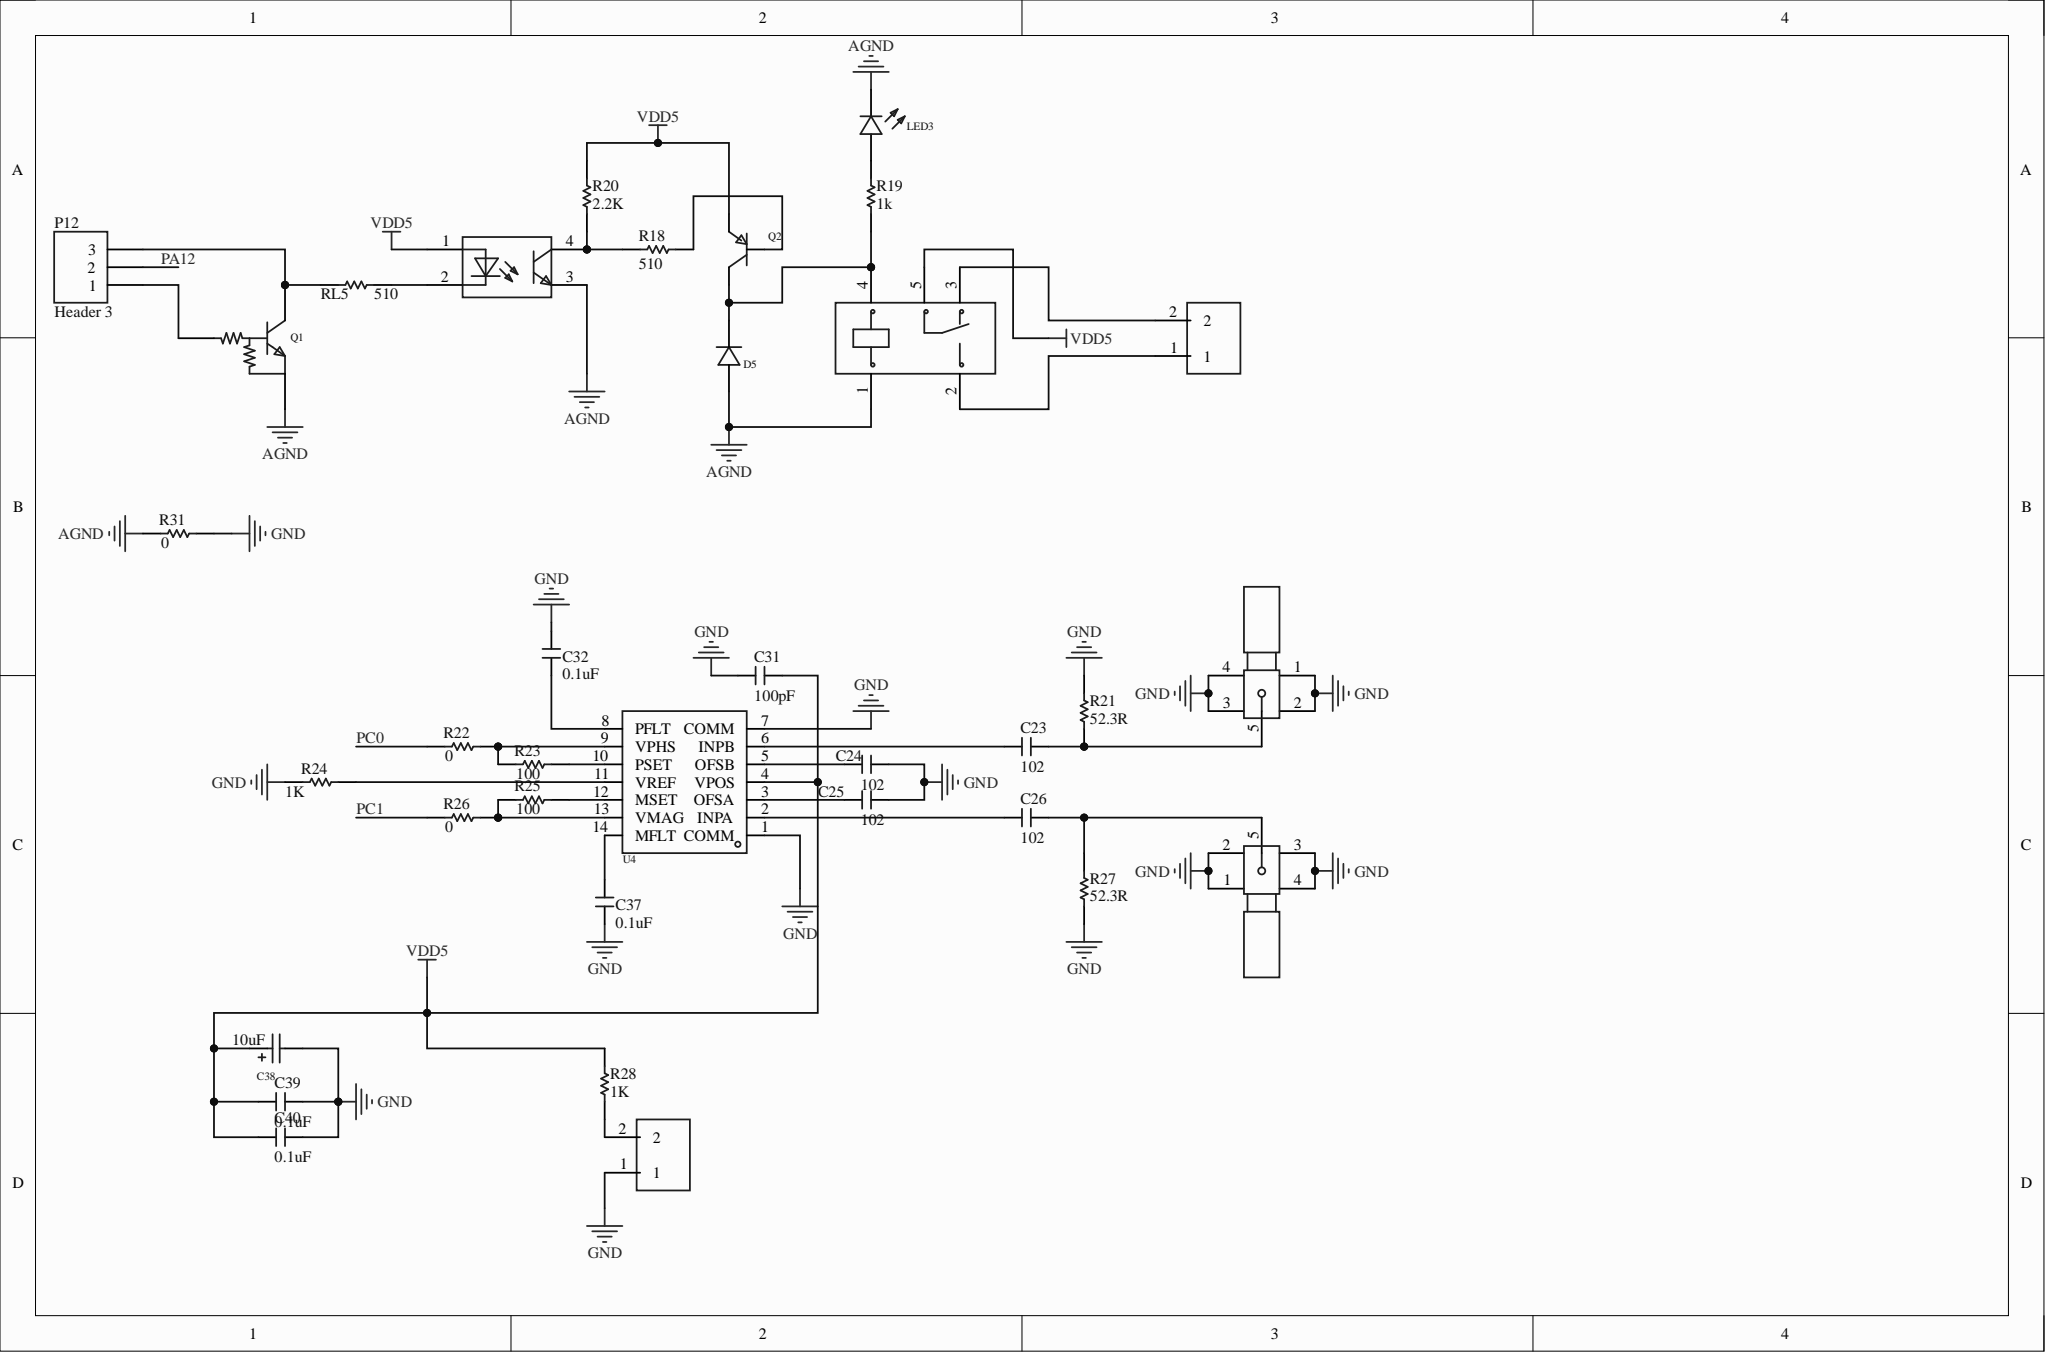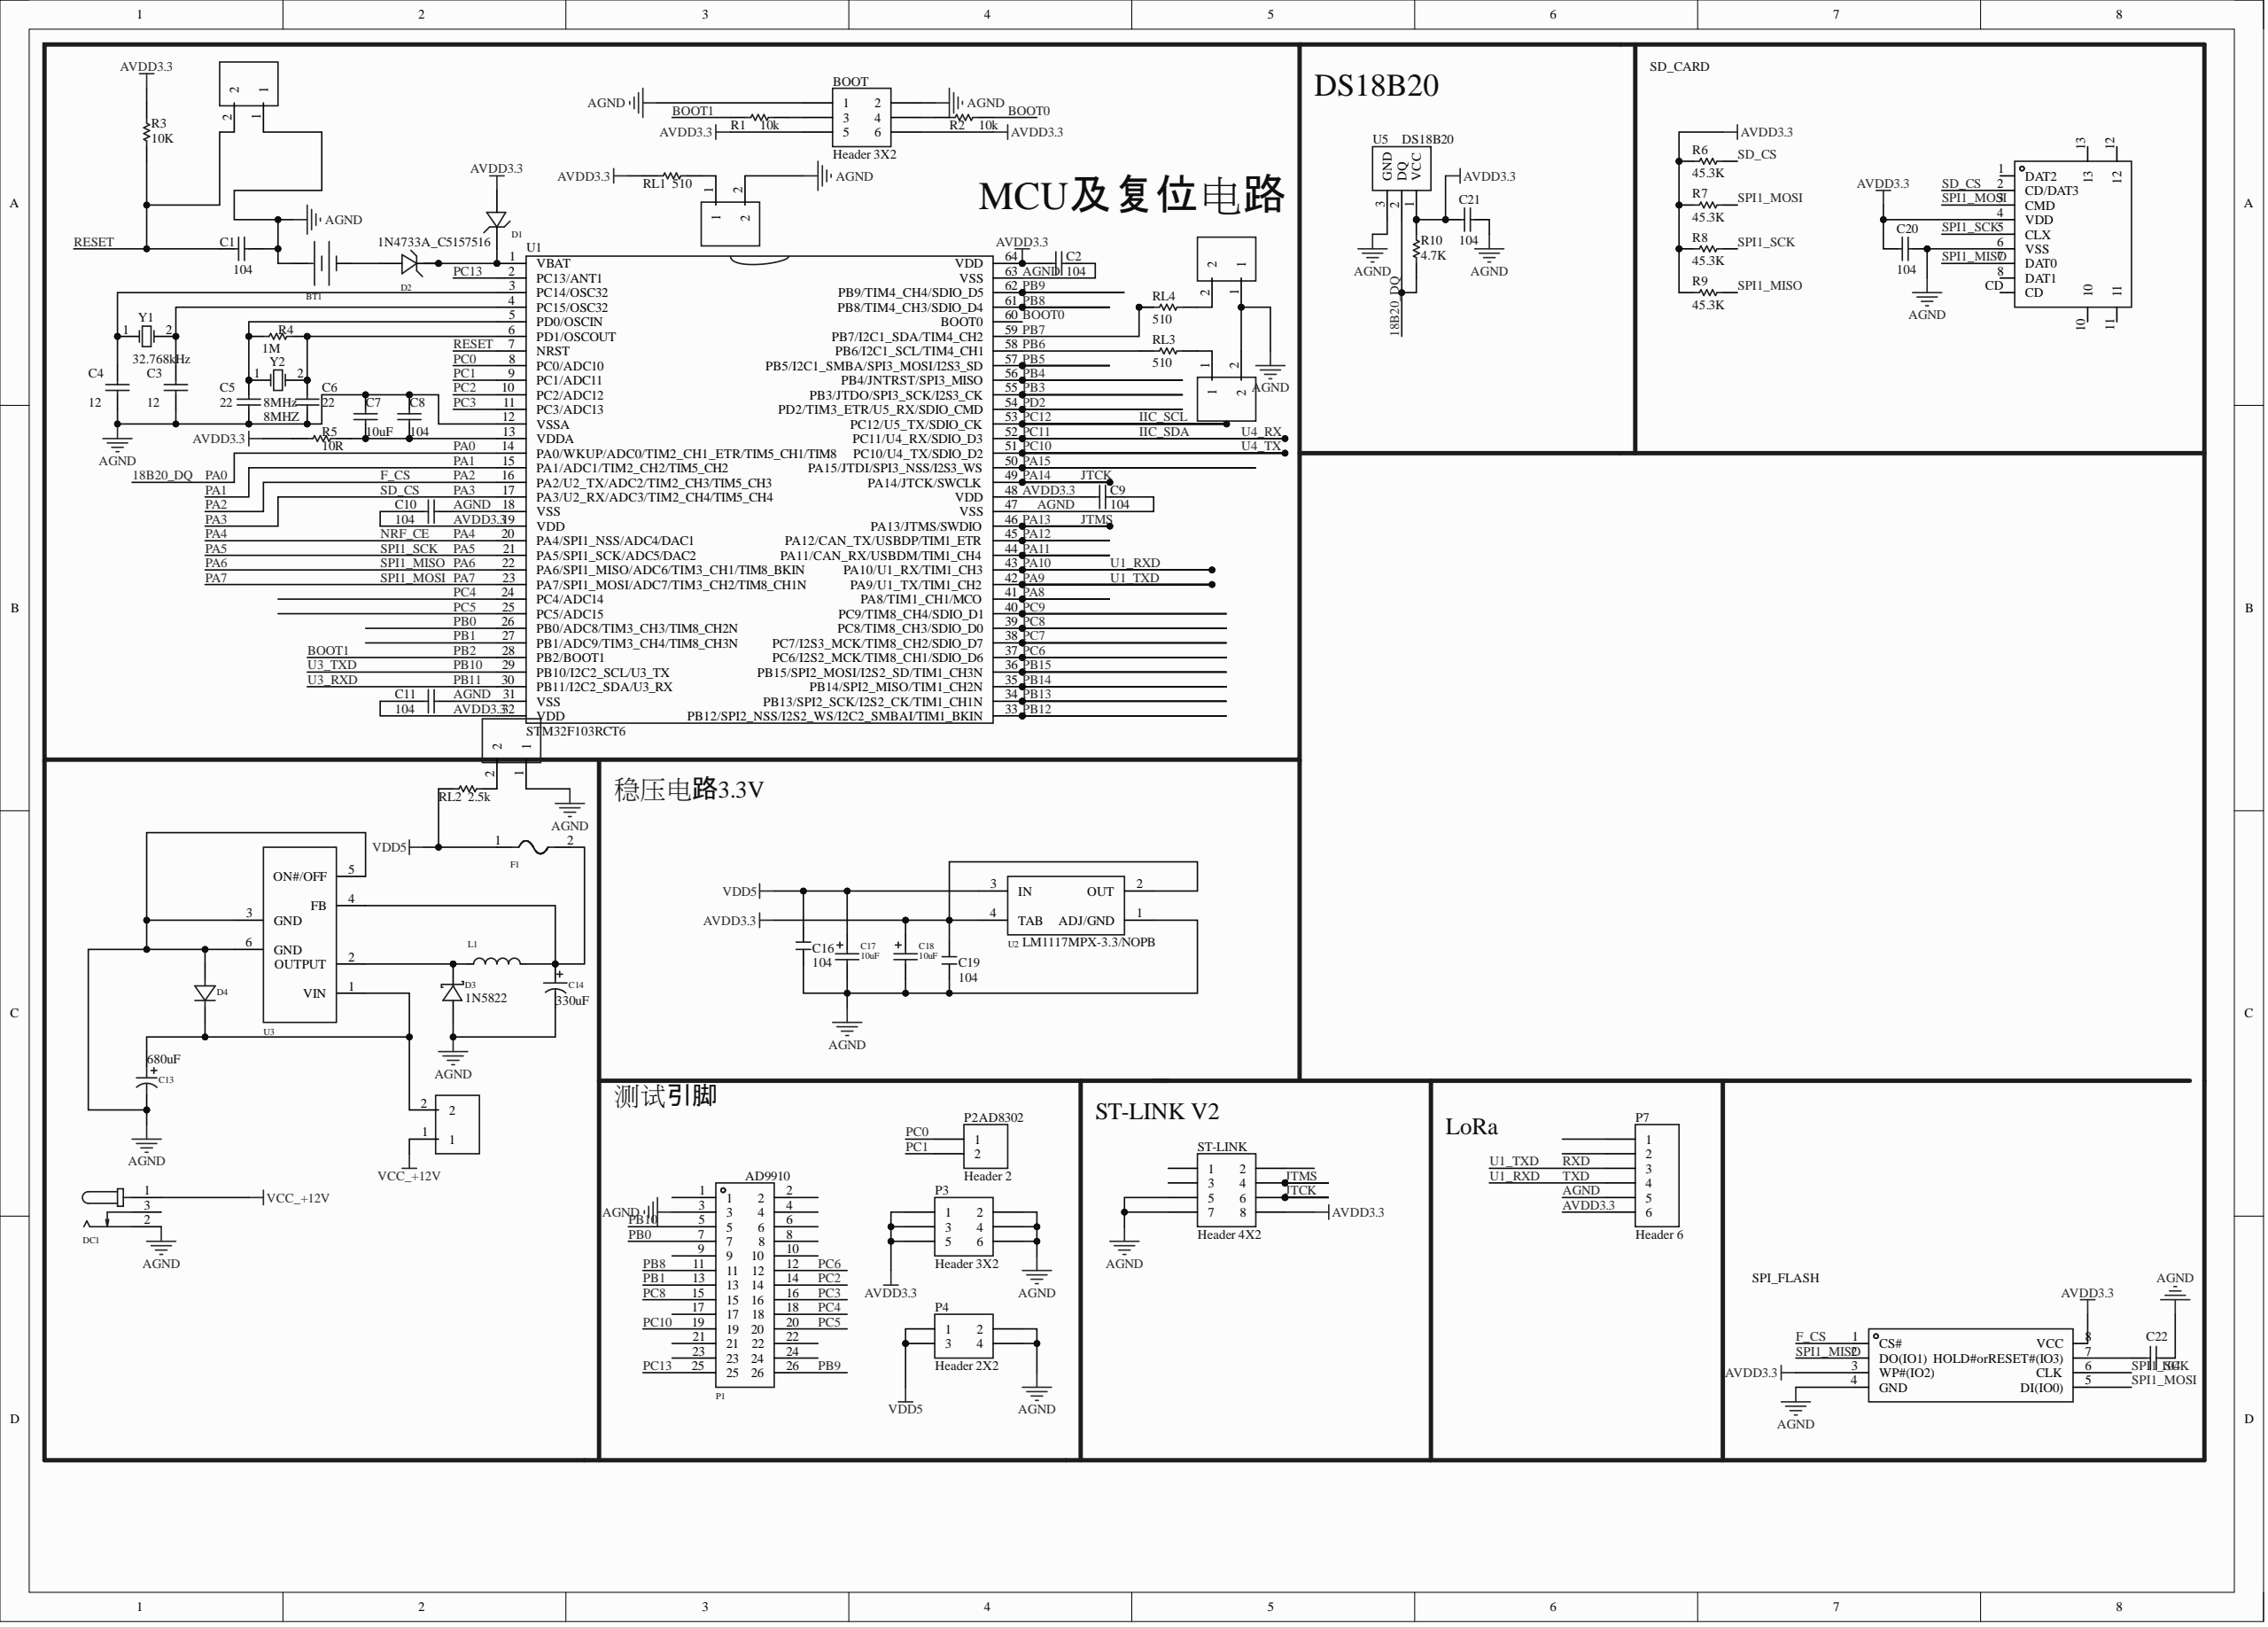Circuit board | Altium Designer | 98 parts | 76 nets
Bill of materials:
Comment,Description,Designator,Footprint,LibRef,Quantity
"Header 3X2","Header, 3-Pin, Dual row","BOOT, P3","HDR2X3","Header 3X2, Header 3X2_1","2"
"BS-12-B3AA003","","BT1","BAT-SMD_BS-12-B3AA011","BS-12-B3AA003","1"
"104","104","C1, C2, C8, C9, C10, C11, C16, C19","C0603","104, 104_1","8"
"12pF","12pF","C3, C4","C0603","12pF","2"
"22pF","22pF","C5, C6","C0603","22pF","2"
"10uF","10uF","C7","C0603","10uF","1"
"GVM1V681M1010","680uF","C13","CAP-SMD_BD10.0-L10.3-W10.3-LS10.9-FD","GVM1V681M1010","1"
"EEEFK1V331P","330uF","C14","CAP-SMD_BD10.0-L10.3-W10.3-FD","EEEFK1V331P","1"
"TAJA106K016RNJ","10uF","C17, C18","CAP-SMD_L3.2-W1.6-RD-C7171","TAJA106K016RNJ","2"
"Cap","104, Cap","C20, C21, C22","CAP[0603]","Cap","3"
"102","102","C23, C24, C25, C26","C0603","102","4"
"100pF","100pF","C31","C0603","100pF","1"
"0.1uF","0.1uF","C32, C37, C39, C40","C0603","0.1uF","4"
"10uF","10uF","C38","CAP-SMD_L3.2-W1.6-RD-C7171","10uF_1","1"
"TF PUSH","","CARD","TF-SMD_TF-PUSH","TF PUSH","1"
"1N4733A_C5157516","","D1, D2","DO-41_BD2.4-L4.7-P8.70-D0.9-RD","1N4733A_C5157516","2"
"1N5822","","D3","DO-201AD_BD5.3-L8.4-P12.50-D1.4-FD","1N5822","1"
"1N4007_C727081","","D4","SMA_L4.3-W2.5-LS5.0-RD","1N4007_C727081","1"
"1N4007W","","D5","SOD-123FL_L2.7-W1.8-LS3.8-RD","1N4007W","1"
"DC-005-20A_C136744","","DC1","DC-IN-TH_DC-005-20A","DC-005-20A_C136744","1"
"BSMD1812-150-33V","","F1","F1812","BSMD1812-150-33V","1"
"FXL0650-330-M","","L1","IND-SMD_L7.0-W6.6_FXL0650","FXL0650-330-M","1"
"NCD0603R1_C84263","","LED3","LED0603-RD_RED","NCD0603R1_C84263","1"
"X1270WV-2x13A-6TV01","","P1","IDC-TH_X1270WV-2X13A-6TV01","X1270WV-2x13A-6TV01","1"
"Header 2","Header, 2-Pin","P2","HDR1X2","Header 2","1"
"Header 2X2","Header, 2-Pin, Dual row","P4","HDR2X2","Header 2X2","1"
"Header 6","Header, 6-Pin","P7","HDR1X6","Header 6","1"
"Header 3","Header, 3-Pin","P12","HDR1X3","Header 3","1"
"WJ126V-5.0-2P","","P13, P17, P18, P19, P20, P21, P22, P23","CONN-TH_WJ126V-5.0-2P","WJ126V-5.0-2P_1, WJ126V-5.0-2P","8"
"DTC143ECA","","Q1","SOT-23-3_L2.9-W1.6-P1.90-LS2.8-BR","DTC143ECA","1"
"MMBT3906","","Q2","SOT-23-3_L2.9-W1.3-P1.90-LS2.4-BR","MMBT3906","1"
"10k","10K, Res","R1, R18, R19, R20","R0603 - duplicate","10k_1","4"
"10k","10K","R2, R3","R0603","10k","2"
"1M","Res","R4","R0603","1M","1"
"10R","10","R5","R0603","10R","1"
"Res","45.3K, 4.7K","R6, R7, R8, R9, R10","RES[0603]","Res","5"
"52.3R","52.3R","R21, R27","R0603","52.3R","2"
"0","0","R22, R26, R31","R0603","0","3"
"100","100","R23, R25","R0603","100","2"
"1K","1K","R24, R28","R0603","1K","2"
"BWSMA-KWE-Z001","","RF1, RF?1","SMA-TH_BWSMA-KWE-Z001","BWSMA-KWE-Z001_1, BWSMA-KWE-Z001","2"
"330","510, 2.5K, Res","RL1, RL2, RL3, RL4, RL5","R0603 - duplicate","330","5"
"SRD-05VDC-SL-C","","RLY1","RELAY-TH_SRD-XXVDC-XL-C","SRD-05VDC-SL-C","1"
"Header 4X2","Header, 4-Pin, Dual row","ST-LINK","HDR2X4","Header 4X2","1"
"STM32F103RCT6","","U1","TQFP-64_L10.0-W10.0-P0.50-LS12.0-BL","STM32F103RCT6","1"
"LM1117MPX-3.3/NOPB","","U2","SOT-223-3_L6.5-W3.4-P2.30-LS7.0-BR","LM1117MPX-3.3/NOPB","1"
"LM2596SX-5.0/NOPB","","U3","TO-263-5_L10.2-W8.9-P1.70-TL","LM2596SX-5.0/NOPB","1"
"AD8302ARUZ-RL7","","U4","TSSOP-14_L5.0-W4.4-P0.65-LS6.4-BL","AD8302ARUZ-RL7","1"
"DS18B20","DS18B20","U5","H2.54-1X3(RM)","DS18B20","1"
"BPC-817SC","","U6","OPTO-SMD-4_L4.6-W6.5-P2.54-LS10.3-BR","BPC-817SC","1"
"W25Q64JVSSIQ","","W25Q64","SOIC-8_L5.3-W5.3-P1.27-LS8.0-BL","W25Q64JVSSIQ","1"
"32.768kHz","XTAL","Y1","OSC-TH_BD2.0-P0.70-D0.3","32.768kHz","1"
"8MHz","XTAL","Y2","OSC-TH_L11.1-W4.7-P4.88","8MHz","1"
Netlist (Protel format):
[
BOOT
HDR2X3
Header 3X2



]
[
BT1
BAT-SMD_BS-12-B3AA011
BS-12-B3AA003



]
[
C1
C0603
104



]
[
C2
C0603
104



]
[
C3
C0603
12pF



]
[
C4
C0603
12pF



]
[
C5
C0603
22pF



]
[
C6
C0603
22pF



]
[
C7
C0603
10uF



]
[
C8
C0603
104



]
[
C9
C0603
104



]
[
C10
C0603
104



]
[
C11
C0603
104



]
[
C13
CAP-SMD_BD10.0-L10.3-W10.3-LS10.9-FD
GVM1V681M1010



]
[
C14
CAP-SMD_BD10.0-L10.3-W10.3-FD
EEEFK1V331P



]
[
C16
C0603
104



]
[
C17
CAP-SMD_L3.2-W1.6-RD-C7171
TAJA106K016RNJ



]
[
C18
CAP-SMD_L3.2-W1.6-RD-C7171
TAJA106K016RNJ



]
[
C19
C0603
104



]
[
C20
CAP[0603]
Cap



]
[
C21
CAP[0603]
Cap



]
[
C22
CAP[0603]
Cap



]
[
C23
C0603
102



]
[
C24
C0603
102



]
[
C25
C0603
102



]
[
C26
C0603
102



]
[
C31
C0603
100pF



]
[
C32
C0603
0.1uF



]
[
C37
C0603
0.1uF



]
[
C38
CAP-SMD_L3.2-W1.6-RD-C7171
10uF



]
[
C39
C0603
0.1uF



]
[
C40
C0603
0.1uF



]
[
CARD
TF-SMD_TF-PUSH
TF PUSH



]
[
D1
DO-41_BD2.4-L4.7-P8.70-D0.9-RD
1N4733A_C5157516



]
[
D2
DO-41_BD2.4-L4.7-P8.70-D0.9-RD
1N4733A_C5157516



]
[
D3
DO-201AD_BD5.3-L8.4-P12.50-D1.4-FD
1N5822



]
[
D4
SMA_L4.3-W2.5-LS5.0-RD
1N4007_C727081



]
[
D5
SOD-123FL_L2.7-W1.8-LS3.8-RD
1N4007W



]
[
DC1
DC-IN-TH_DC-005-20A
DC-005-20A_C136744



]
[
F1
F1812
BSMD1812-150-33V



]
[
L1
IND-SMD_L7.0-W6.6_FXL0650
FXL0650-330-M



]
[
LED3
LED0603-RD_RED
NCD0603R1_C84263



]
[
P1
IDC-TH_X1270WV-2X13A-6TV01
X1270WV-2x13A-6TV01



]
[
P2
HDR1X2
Header 2



]
[
P3
HDR2X3
Header 3X2



]
[
P4
HDR2X2
Header 2X2



]
[
P7
HDR1X6
Header 6



]
[
P12
HDR1X3
Header 3



]
[
P13
CONN-TH_WJ126V-5.0-2P
WJ126V-5.0-2P



]
[
P17
CONN-TH_WJ126V-5.0-2P
WJ126V-5.0-2P



]
[
P18
CONN-TH_WJ126V-5.0-2P
WJ126V-5.0-2P



]
[
P19
CONN-TH_WJ126V-5.0-2P
WJ126V-5.0-2P



]
[
P20
CONN-TH_WJ126V-5.0-2P
WJ126V-5.0-2P



]
[
P21
CONN-TH_WJ126V-5.0-2P
WJ126V-5.0-2P



]
[
P22
CONN-TH_WJ126V-5.0-2P
WJ126V-5.0-2P



]
[
P23
CONN-TH_WJ126V-5.0-2P
WJ126V-5.0-2P



]
[
Q1
SOT-23-3_L2.9-W1.6-P1.90-LS2.8-BR
DTC143ECA



]
[
Q2
SOT-23-3_L2.9-W1.3-P1.90-LS2.4-BR
MMBT3906



]
[
R1
R0603 - duplicate
10k



]
[
R2
R0603
10k



]
[
R3
R0603
10k



]
[
R4
R0603
1M



]
[
R5
R0603
10R



]
[
R6
RES[0603]
Res



]
[
R7
RES[0603]
Res



]
[
R8
RES[0603]
Res



]
[
R9
RES[0603]
Res



]
[
R10
RES[0603]
Res



]
[
R18
R0603 - duplicate
10k



]
[
R19
R0603 - duplicate
10k



]
[
R20
R0603 - duplicate
10k



]
[
R21
R0603
52.3R



]
[
R22
R0603
0



]
[
R23
R0603
100



]
[
R24
R0603
1K



]
[
R25
R0603
100



]
[
R26
R0603
0



]
[
R27
R0603
52.3R



]
[
R28
R0603
1K



]
[
R31
R0603
0



]
[
RF1
SMA-TH_BWSMA-KWE-Z001
BWSMA-KWE-Z001



]
[
RF?1
SMA-TH_BWSMA-KWE-Z001
BWSMA-KWE-Z001



]
[
RL1
R0603 - duplicate
330



]
[
RL2
R0603 - duplicate
330



]
[
RL3
R0603 - duplicate
330



]
[
RL4
R0603 - duplicate
330



]
[
RL5
R0603 - duplicate
330



]
[
RLY1
RELAY-TH_SRD-XXVDC-XL-C
SRD-05VDC-SL-C



]
[
ST-LINK
HDR2X4
Header 4X2



]
[
U1
TQFP-64_L10.0-W10.0-P0.50-LS12.0-BL
STM32F103RCT6



]
[
U2
SOT-223-3_L6.5-W3.4-P2.30-LS7.0-BR
LM1117MPX-3.3/NOPB



]
[
U3
TO-263-5_L10.2-W8.9-P1.70-TL
LM2596SX-5.0/NOPB



]
[
U4
TSSOP-14_L5.0-W4.4-P0.65-LS6.4-BL
AD8302ARUZ-RL7



]
[
U5
H2.54-1X3(RM)
DS18B20



]
[
U6
OPTO-SMD-4_L4.6-W6.5-P2.54-LS10.3-BR
BPC-817SC



]
[
W25Q64
SOIC-8_L5.3-W5.3-P1.27-LS8.0-BL
W25Q64JVSSIQ



]
[
Y1
OSC-TH_BD2.0-P0.70-D0.3
32.768kHz



]
[
Y2
OSC-TH_L11.1-W4.7-P4.88
8MHz



]
(
VDD5
C16-2
C17-1
C31-1
C38-1
C39-2
C40-2
F1-1
P4-1
P4-3
Q2-2
R20-1
R28-2
RL2-1
RLY1-5
U2-3
U4-4
U6-1
)
(
VCC_+12V
DC1-1
P22-1
)
(
RESET
C1-1
P23-2
R3-1
U1-7
)
(
PC13
P1-25
U1-2
)
(
PC10
P1-19
U1-51
)
(
PC8
P1-15
U1-39
)
(
PC6
P1-12
U1-37
)
(
PC5
P1-20
U1-25
)
(
PC4
P1-18
U1-24
)
(
PC3
P1-16
U1-11
)
(
PC2
P1-14
U1-10
)
(
PC1
P2-2
R26-1
U1-9
)
(
PC0
P2-1
R22-1
U1-8
)
(
PB10
P1-5
U1-29
)
(
PB9
P1-26
U1-62
)
(
PB8
P1-11
U1-61
)
(
PB7
RL4-2
U1-59
)
(
PB6
RL3-2
U1-58
)
(
PB1
P1-13
U1-27
)
(
PB0
P1-7
U1-26
)
(
PA12
P12-2
U1-45
)
(
PA10
P7-4
U1-43
)
(
PA9
P7-3
U1-42
)
(
PA7
CARD-3
R7-2
U1-23
W25Q64-5
)
(
PA6
CARD-7
R9-2
U1-22
W25Q64-2
)
(
PA5
CARD-5
R8-2
U1-21
W25Q64-6
)
(
PA3
CARD-2
R6-2
U1-17
)
(
NetRL5_2
RL5-2
U6-2
)
(
NetR25_2
R25-2
U4-12
)
(
NetR25_1
R25-1
R26-2
U4-13
)
(
NetR24_2
R24-2
U4-11
)
(
NetR23_2
R23-2
U4-10
)
(
NetR22_2
R22-2
R23-1
U4-9
)
(
NetR18_1
R18-1
R20-2
U6-4
)
(
NetQ2_1
Q2-1
R18-2
)
(
NetP21_2
P21-2
RL2-2
)
(
NetP20_1
P20-1
RL1-2
)
(
NetP19_1
P19-1
RL3-1
)
(
NetP18_2
P18-2
RL4-1
)
(
NetP17_2
P17-2
R28-1
)
(
NetP13_2
P13-2
RLY1-3
)
(
NetP13_1
P13-1
RLY1-2
)
(
NetP12_3
P12-3
Q1-3
RL5-1
)
(
NetP12_1
P12-1
Q1-1
)
(
NetLED3_2
LED3-2
R19-1
)
(
NetD5_1
D5-1
Q2-3
R19-2
RLY1-4
)
(
NetD3_2
D3-2
L1-1
U3-2
)
(
NetD1_1
D1-1
D2-1
U1-1
)
(
NetC37_2
C37-2
U4-14
)
(
NetC32_1
C32-1
U4-8
)
(
NetC26_2
C26-2
U4-2
)
(
NetC26_1
C26-1
R27-2
RF?1-5
)
(
NetC25_2
C25-2
U4-3
)
(
NetC24_2
C24-2
U4-5
)
(
NetC23_2
C23-2
U4-6
)
(
NetC23_1
C23-1
R21-1
RF1-5
)
(
NetC22_1
C22-1
W25Q64-7
)
(
NetC14_1
C14-1
F1-2
L1-2
U3-4
)
(
NetC13_1
C13-1
D4-1
P22-2
U3-1
)
(
NetC7_1
C7-1
C8-1
R5-1
U1-13
)
(
NetC6_2
C6-2
R4-1
U1-6
Y2-2
)
(
NetC5_2
C5-2
R4-2
U1-5
Y2-1
)
(
NetC4_2
C4-2
U1-3
Y1-1
)
(
NetC3_2
C3-2
U1-4
Y1-2
)
(
NetBT1_2
BT1-2
D2-2
)
(
NetBOOT_4
BOOT-4
R2-1
)
(
NetBOOT_3
BOOT-3
R1-2
)
(
JTMS
ST-LINK-4
U1-46
)
(
JTCK
ST-LINK-6
U1-49
)
(
GND
C24-1
C25-1
C31-2
C32-2
C37-1
C38-2
C39-1
C40-1
P17-1
R21-2
R24-1
R27-1
R31-2
RF1-1
RF1-2
RF1-3
RF1-4
RF?1-1
RF?1-2
RF?1-3
RF?1-4
U4-1
U4-7
)
(
F_CS
U1-16
W25Q64-1
)
(
BOOT1
R1-1
U1-28
)
(
BOOT0
R2-2
U1-60
)
(
AVDD3.3
BOOT-5
BOOT-6
C2-1
C9-1
C10-2
C11-2
C18-1
C19-2
C20-1
C21-1
CARD-4
D1-2
P3-1
P3-3
P3-5
P7-6
R3-2
R5-2
R6-1
R7-1
R8-1
R9-1
R10-2
RL1-1
ST-LINK-8
U1-19
U1-32
U1-48
U1-64
U2-2
U2-4
U5-1
W25Q64-3
W25Q64-8
)
(
AGND
BOOT-1
BOOT-2
BT1-1
C1-2
C2-2
C3-1
C4-1
C5-1
C6-1
C7-2
C8-2
C9-2
C10-1
C11-1
C13-2
C14-2
C16-1
C17-2
C18-2
C19-1
C20-2
C21-2
C22-2
CARD-6
D3-1
D4-2
D5-2
DC1-2
LED3-1
P1-3
P3-2
P3-4
P3-6
P4-2
P4-4
P7-5
P18-1
P19-2
P20-2
P21-1
P23-1
Q1-2
R31-1
RLY1-1
ST-LINK-5
ST-LINK-7
U1-12
U1-18
U1-31
U1-47
U1-63
U2-1
U3-3
U3-5
U3-6
U5-3
U6-3
W25Q64-4
)
(
18B20_DQ
R10-1
U1-14
U5-2
)